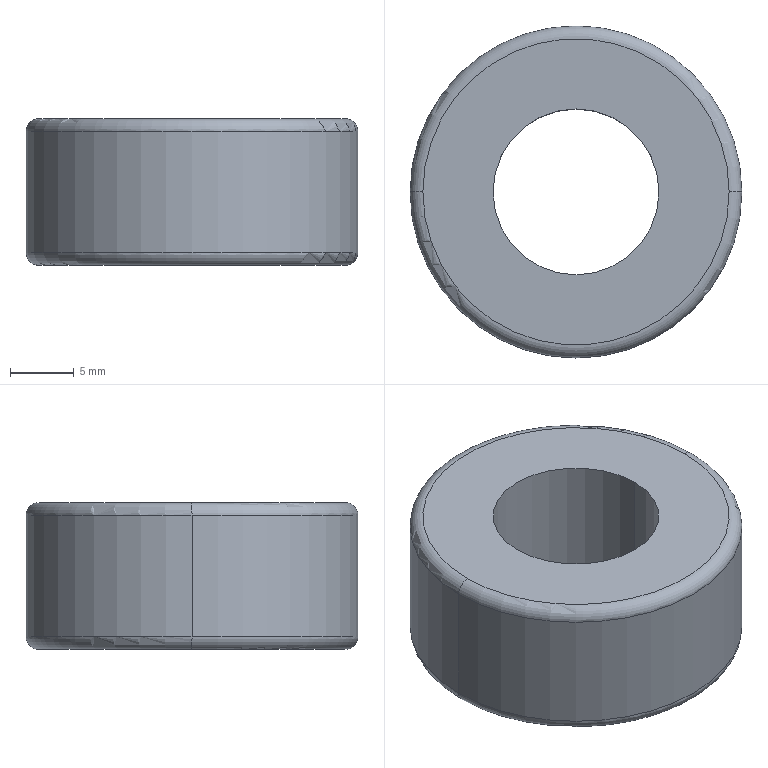Part | SolidWorks | features Extrusion 1, Fillet 1 | 1 solid | 10 faces | box 26 x 26 x 11.5 mm | volume 4545 mm3 | torus 4 | cylinder 4 | plane 2 | commonest cylinder face diameters 13 x2 26 x2
STEP:
#1=CARTESIAN_POINT('',(-13.,0.,10.5));
#2=VERTEX_POINT('',#1);
#3=CARTESIAN_POINT('',(13.,0.,10.5));
#4=VERTEX_POINT('',#3);
#5=CARTESIAN_POINT('',(0.,0.,10.5));
#6=DIRECTION('',(0.,0.,-1.));
#7=DIRECTION('',(1.,0.,0.));
#8=AXIS2_PLACEMENT_3D('',#5,#6,#7);
#9=CIRCLE('',#8,13.);
#10=EDGE_CURVE('',#2,#4,#9,.T.);
#11=ORIENTED_EDGE('',*,*,#10,.F.);
#12=CARTESIAN_POINT('',(-12.,0.,11.5));
#13=VERTEX_POINT('',#12);
#14=CARTESIAN_POINT('',(-12.,0.,10.5));
#15=DIRECTION('',(0.,1.,0.));
#16=DIRECTION('',(-1.,0.,0.));
#17=AXIS2_PLACEMENT_3D('',#14,#15,#16);
#18=CIRCLE('',#17,1.);
#19=EDGE_CURVE('',#2,#13,#18,.T.);
#20=ORIENTED_EDGE('',*,*,#19,.T.);
#21=CARTESIAN_POINT('',(12.,0.,11.5));
#22=VERTEX_POINT('',#21);
#23=CARTESIAN_POINT('',(0.,0.,11.5));
#24=DIRECTION('',(0.,0.,1.));
#25=DIRECTION('',(1.,0.,0.));
#26=AXIS2_PLACEMENT_3D('',#23,#24,#25);
#27=CIRCLE('',#26,12.);
#28=EDGE_CURVE('',#22,#13,#27,.T.);
#29=ORIENTED_EDGE('',*,*,#28,.F.);
#30=CARTESIAN_POINT('',(12.,0.,10.5));
#31=DIRECTION('',(0.,-1.,0.));
#32=DIRECTION('',(0.,0.,-1.));
#33=AXIS2_PLACEMENT_3D('',#30,#31,#32);
#34=CIRCLE('',#33,1.);
#35=EDGE_CURVE('',#4,#22,#34,.T.);
#36=ORIENTED_EDGE('',*,*,#35,.F.);
#37=EDGE_LOOP('',(#11,#20,#29,#36));
#38=FACE_OUTER_BOUND('',#37,.T.);
#39=CARTESIAN_POINT('',(0.,0.,10.5));
#40=DIRECTION('',(0.,0.,1.));
#41=DIRECTION('',(1.,0.,0.));
#42=AXIS2_PLACEMENT_3D('',#39,#40,#41);
#43=TOROIDAL_SURFACE('',#42,12.,1.);
#44=ADVANCED_FACE('',(#38),#43,.T.);
#45=CARTESIAN_POINT('',(-12.,0.,0.));
#46=VERTEX_POINT('',#45);
#47=CARTESIAN_POINT('',(12.,0.,0.));
#48=VERTEX_POINT('',#47);
#49=CARTESIAN_POINT('',(0.,0.,0.));
#50=DIRECTION('',(0.,0.,-1.));
#51=DIRECTION('',(1.,0.,0.));
#52=AXIS2_PLACEMENT_3D('',#49,#50,#51);
#53=CIRCLE('',#52,12.);
#54=EDGE_CURVE('',#46,#48,#53,.T.);
#55=ORIENTED_EDGE('',*,*,#54,.F.);
#56=CARTESIAN_POINT('',(-13.,0.,1.));
#57=VERTEX_POINT('',#56);
#58=CARTESIAN_POINT('',(-12.,0.,1.));
#59=DIRECTION('',(0.,1.,0.));
#60=DIRECTION('',(-1.,0.,0.));
#61=AXIS2_PLACEMENT_3D('',#58,#59,#60);
#62=CIRCLE('',#61,1.);
#63=EDGE_CURVE('',#46,#57,#62,.T.);
#64=ORIENTED_EDGE('',*,*,#63,.T.);
#65=CARTESIAN_POINT('',(13.,0.,1.));
#66=VERTEX_POINT('',#65);
#67=CARTESIAN_POINT('',(0.,0.,1.));
#68=DIRECTION('',(0.,0.,1.));
#69=DIRECTION('',(1.,0.,0.));
#70=AXIS2_PLACEMENT_3D('',#67,#68,#69);
#71=CIRCLE('',#70,13.);
#72=EDGE_CURVE('',#66,#57,#71,.T.);
#73=ORIENTED_EDGE('',*,*,#72,.F.);
#74=CARTESIAN_POINT('',(12.,0.,1.));
#75=DIRECTION('',(0.,-1.,0.));
#76=DIRECTION('',(0.,0.,-1.));
#77=AXIS2_PLACEMENT_3D('',#74,#75,#76);
#78=CIRCLE('',#77,1.);
#79=EDGE_CURVE('',#48,#66,#78,.T.);
#80=ORIENTED_EDGE('',*,*,#79,.F.);
#81=EDGE_LOOP('',(#55,#64,#73,#80));
#82=FACE_OUTER_BOUND('',#81,.T.);
#83=CARTESIAN_POINT('',(0.,0.,1.));
#84=DIRECTION('',(0.,0.,1.));
#85=DIRECTION('',(1.,0.,0.));
#86=AXIS2_PLACEMENT_3D('',#83,#84,#85);
#87=TOROIDAL_SURFACE('',#86,12.,1.);
#88=ADVANCED_FACE('',(#82),#87,.T.);
#89=CARTESIAN_POINT('',(-6.5,0.,11.5));
#90=VERTEX_POINT('',#89);
#91=CARTESIAN_POINT('',(6.5,0.,11.5));
#92=VERTEX_POINT('',#91);
#93=CARTESIAN_POINT('',(0.,0.,11.5));
#94=DIRECTION('',(0.,0.,1.));
#95=DIRECTION('',(1.,0.,0.));
#96=AXIS2_PLACEMENT_3D('',#93,#94,#95);
#97=CIRCLE('',#96,6.5);
#98=EDGE_CURVE('',#90,#92,#97,.T.);
#99=ORIENTED_EDGE('',*,*,#98,.T.);
#100=CARTESIAN_POINT('',(6.5,0.,0.));
#101=VERTEX_POINT('',#100);
#102=CARTESIAN_POINT('',(6.5,0.,11.5));
#103=DIRECTION('',(0.,0.,-1.));
#104=VECTOR('',#103,1000.);
#105=LINE('',#102,#104);
#106=EDGE_CURVE('',#92,#101,#105,.T.);
#107=ORIENTED_EDGE('',*,*,#106,.T.);
#108=CARTESIAN_POINT('',(-6.5,0.,0.));
#109=VERTEX_POINT('',#108);
#110=CARTESIAN_POINT('',(0.,0.,0.));
#111=DIRECTION('',(0.,0.,1.));
#112=DIRECTION('',(1.,0.,0.));
#113=AXIS2_PLACEMENT_3D('',#110,#111,#112);
#114=CIRCLE('',#113,6.5);
#115=EDGE_CURVE('',#109,#101,#114,.T.);
#116=ORIENTED_EDGE('',*,*,#115,.F.);
#117=CARTESIAN_POINT('',(-6.5,0.,11.5));
#118=DIRECTION('',(0.,0.,-1.));
#119=VECTOR('',#118,1000.);
#120=LINE('',#117,#119);
#121=EDGE_CURVE('',#90,#109,#120,.T.);
#122=ORIENTED_EDGE('',*,*,#121,.F.);
#123=EDGE_LOOP('',(#99,#107,#116,#122));
#124=FACE_OUTER_BOUND('',#123,.T.);
#125=CARTESIAN_POINT('',(0.,0.,11.5));
#126=DIRECTION('',(0.,0.,-1.));
#127=DIRECTION('',(-1.,0.,0.));
#128=AXIS2_PLACEMENT_3D('',#125,#126,#127);
#129=CYLINDRICAL_SURFACE('',#128,6.5);
#130=ADVANCED_FACE('',(#124),#129,.F.);
#131=ORIENTED_EDGE('',*,*,#10,.T.);
#132=CARTESIAN_POINT('',(13.,0.,11.5));
#133=DIRECTION('',(0.,0.,-1.));
#134=VECTOR('',#133,1000.);
#135=LINE('',#132,#134);
#136=EDGE_CURVE('',#4,#66,#135,.T.);
#137=ORIENTED_EDGE('',*,*,#136,.T.);
#138=ORIENTED_EDGE('',*,*,#72,.T.);
#139=CARTESIAN_POINT('',(-13.,0.,11.5));
#140=DIRECTION('',(0.,0.,-1.));
#141=VECTOR('',#140,1000.);
#142=LINE('',#139,#141);
#143=EDGE_CURVE('',#2,#57,#142,.T.);
#144=ORIENTED_EDGE('',*,*,#143,.F.);
#145=EDGE_LOOP('',(#131,#137,#138,#144));
#146=FACE_OUTER_BOUND('',#145,.T.);
#147=CARTESIAN_POINT('',(0.,0.,11.5));
#148=DIRECTION('',(0.,0.,-1.));
#149=DIRECTION('',(-1.,0.,0.));
#150=AXIS2_PLACEMENT_3D('',#147,#148,#149);
#151=CYLINDRICAL_SURFACE('',#150,13.);
#152=ADVANCED_FACE('',(#146),#151,.T.);
#153=ORIENTED_EDGE('',*,*,#28,.T.);
#154=CARTESIAN_POINT('',(0.,0.,11.5));
#155=DIRECTION('',(0.,0.,1.));
#156=DIRECTION('',(1.,0.,0.));
#157=AXIS2_PLACEMENT_3D('',#154,#155,#156);
#158=CIRCLE('',#157,12.);
#159=EDGE_CURVE('',#13,#22,#158,.T.);
#160=ORIENTED_EDGE('',*,*,#159,.T.);
#161=EDGE_LOOP('',(#153,#160));
#162=FACE_OUTER_BOUND('',#161,.T.);
#163=ORIENTED_EDGE('',*,*,#98,.F.);
#164=CARTESIAN_POINT('',(0.,0.,11.5));
#165=DIRECTION('',(0.,0.,1.));
#166=DIRECTION('',(1.,0.,0.));
#167=AXIS2_PLACEMENT_3D('',#164,#165,#166);
#168=CIRCLE('',#167,6.5);
#169=EDGE_CURVE('',#92,#90,#168,.T.);
#170=ORIENTED_EDGE('',*,*,#169,.F.);
#171=EDGE_LOOP('',(#163,#170));
#172=FACE_BOUND('',#171,.T.);
#173=CARTESIAN_POINT('',(0.,0.,11.5));
#174=DIRECTION('',(0.,0.,1.));
#175=DIRECTION('',(1.,0.,0.));
#176=AXIS2_PLACEMENT_3D('',#173,#174,#175);
#177=PLANE('',#176);
#178=ADVANCED_FACE('',(#162,#172),#177,.T.);
#179=CARTESIAN_POINT('',(0.,0.,0.));
#180=DIRECTION('',(0.,0.,-1.));
#181=DIRECTION('',(1.,0.,0.));
#182=AXIS2_PLACEMENT_3D('',#179,#180,#181);
#183=CIRCLE('',#182,12.);
#184=EDGE_CURVE('',#48,#46,#183,.T.);
#185=ORIENTED_EDGE('',*,*,#184,.T.);
#186=ORIENTED_EDGE('',*,*,#54,.T.);
#187=EDGE_LOOP('',(#185,#186));
#188=FACE_OUTER_BOUND('',#187,.T.);
#189=ORIENTED_EDGE('',*,*,#115,.T.);
#190=CARTESIAN_POINT('',(0.,0.,0.));
#191=DIRECTION('',(0.,0.,1.));
#192=DIRECTION('',(1.,0.,0.));
#193=AXIS2_PLACEMENT_3D('',#190,#191,#192);
#194=CIRCLE('',#193,6.5);
#195=EDGE_CURVE('',#101,#109,#194,.T.);
#196=ORIENTED_EDGE('',*,*,#195,.T.);
#197=EDGE_LOOP('',(#189,#196));
#198=FACE_BOUND('',#197,.T.);
#199=CARTESIAN_POINT('',(0.,0.,0.));
#200=DIRECTION('',(0.,0.,1.));
#201=DIRECTION('',(1.,0.,0.));
#202=AXIS2_PLACEMENT_3D('',#199,#200,#201);
#203=PLANE('',#202);
#204=ADVANCED_FACE('',(#188,#198),#203,.F.);
#205=ORIENTED_EDGE('',*,*,#136,.F.);
#206=CARTESIAN_POINT('',(0.,0.,10.5));
#207=DIRECTION('',(0.,0.,-1.));
#208=DIRECTION('',(1.,0.,0.));
#209=AXIS2_PLACEMENT_3D('',#206,#207,#208);
#210=CIRCLE('',#209,13.);
#211=EDGE_CURVE('',#4,#2,#210,.T.);
#212=ORIENTED_EDGE('',*,*,#211,.T.);
#213=ORIENTED_EDGE('',*,*,#143,.T.);
#214=CARTESIAN_POINT('',(0.,0.,1.));
#215=DIRECTION('',(0.,0.,1.));
#216=DIRECTION('',(1.,0.,0.));
#217=AXIS2_PLACEMENT_3D('',#214,#215,#216);
#218=CIRCLE('',#217,13.);
#219=EDGE_CURVE('',#57,#66,#218,.T.);
#220=ORIENTED_EDGE('',*,*,#219,.T.);
#221=EDGE_LOOP('',(#205,#212,#213,#220));
#222=FACE_OUTER_BOUND('',#221,.T.);
#223=CARTESIAN_POINT('',(0.,0.,11.5));
#224=DIRECTION('',(0.,0.,-1.));
#225=DIRECTION('',(-1.,0.,0.));
#226=AXIS2_PLACEMENT_3D('',#223,#224,#225);
#227=CYLINDRICAL_SURFACE('',#226,13.);
#228=ADVANCED_FACE('',(#222),#227,.T.);
#229=ORIENTED_EDGE('',*,*,#106,.F.);
#230=ORIENTED_EDGE('',*,*,#169,.T.);
#231=ORIENTED_EDGE('',*,*,#121,.T.);
#232=ORIENTED_EDGE('',*,*,#195,.F.);
#233=EDGE_LOOP('',(#229,#230,#231,#232));
#234=FACE_OUTER_BOUND('',#233,.T.);
#235=CARTESIAN_POINT('',(0.,0.,11.5));
#236=DIRECTION('',(0.,0.,-1.));
#237=DIRECTION('',(-1.,0.,0.));
#238=AXIS2_PLACEMENT_3D('',#235,#236,#237);
#239=CYLINDRICAL_SURFACE('',#238,6.5);
#240=ADVANCED_FACE('',(#234),#239,.F.);
#241=ORIENTED_EDGE('',*,*,#63,.F.);
#242=ORIENTED_EDGE('',*,*,#184,.F.);
#243=ORIENTED_EDGE('',*,*,#79,.T.);
#244=ORIENTED_EDGE('',*,*,#219,.F.);
#245=EDGE_LOOP('',(#241,#242,#243,#244));
#246=FACE_OUTER_BOUND('',#245,.T.);
#247=CARTESIAN_POINT('',(0.,0.,1.));
#248=DIRECTION('',(0.,0.,1.));
#249=DIRECTION('',(1.,0.,0.));
#250=AXIS2_PLACEMENT_3D('',#247,#248,#249);
#251=TOROIDAL_SURFACE('',#250,12.,1.);
#252=ADVANCED_FACE('',(#246),#251,.T.);
#253=ORIENTED_EDGE('',*,*,#19,.F.);
#254=ORIENTED_EDGE('',*,*,#211,.F.);
#255=ORIENTED_EDGE('',*,*,#35,.T.);
#256=ORIENTED_EDGE('',*,*,#159,.F.);
#257=EDGE_LOOP('',(#253,#254,#255,#256));
#258=FACE_OUTER_BOUND('',#257,.T.);
#259=CARTESIAN_POINT('',(0.,0.,10.5));
#260=DIRECTION('',(0.,0.,1.));
#261=DIRECTION('',(1.,0.,0.));
#262=AXIS2_PLACEMENT_3D('',#259,#260,#261);
#263=TOROIDAL_SURFACE('',#262,12.,1.);
#264=ADVANCED_FACE('',(#258),#263,.T.);
#265=CLOSED_SHELL('',(#44,#88,#130,#152,#178,#204,#228,#240,#252,#264));
#266=MANIFOLD_SOLID_BREP('',#265);
#267=CARTESIAN_POINT('',(0.,0.,0.));
#268=DIRECTION('',(0.,0.,1.));
#269=DIRECTION('',(1.,0.,0.));
#270=AXIS2_PLACEMENT_3D('',#267,#268,#269);
#271=(LENGTH_UNIT()NAMED_UNIT(*)SI_UNIT(.MILLI.,.METRE.));
#272=UNCERTAINTY_MEASURE_WITH_UNIT(LENGTH_MEASURE(0.00001),#271,'','');
#273=(NAMED_UNIT(*)PLANE_ANGLE_UNIT()SI_UNIT($,.RADIAN.));
#274=(NAMED_UNIT(*)SI_UNIT($,.STERADIAN.)SOLID_ANGLE_UNIT());
#275=(GEOMETRIC_REPRESENTATION_CONTEXT(3)GLOBAL_UNCERTAINTY_ASSIGNED_CONTEXT((#272))GLOBAL_UNIT_ASSIGNED_CONTEXT((#271,#273,#274))REPRESENTATION_CONTEXT('',''));
#276=ADVANCED_BREP_SHAPE_REPRESENTATION('',(#266,#270),#275);